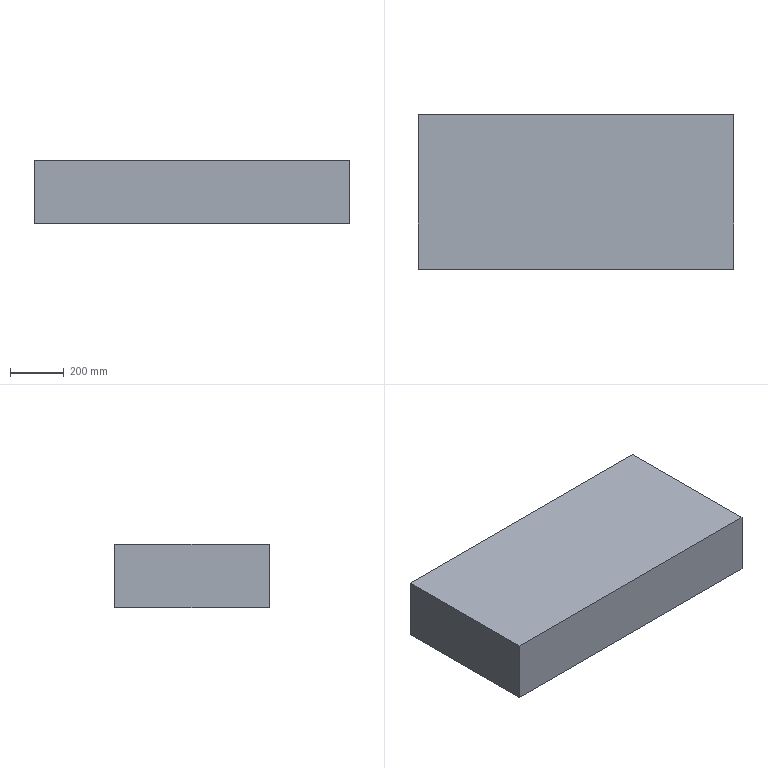Part | STEP file | 复件 Part 1^Upper罩 | 1 solid | 6 faces | box 1175 x 575 x 235 mm | volume 158771875 mm3 | plane 6
STEP:
#1=CARTESIAN_POINT('',(0.,0.,0.));
#2=DIRECTION('',(0.,0.,1.));
#3=DIRECTION('',(1.,0.,0.));
#4=AXIS2_PLACEMENT_3D('',#1,#2,#3);
#5=CARTESIAN_POINT('',(587.5,-287.5,0.));
#6=VERTEX_POINT('',#5);
#7=CARTESIAN_POINT('',(587.5,287.5,0.));
#8=VERTEX_POINT('',#7);
#9=CARTESIAN_POINT('',(587.5,287.5,0.));
#10=DIRECTION('',(0.,1.,0.));
#11=VECTOR('',#10,1.);
#12=LINE('',#9,#11);
#13=CARTESIAN_POINT('',(587.5,287.5,235.));
#14=DIRECTION('',(-1.,0.,0.));
#15=DIRECTION('',(0.,-1.,0.));
#16=AXIS2_PLACEMENT_3D('',#13,#14,#15);
#17=PLANE('',#16);
#18=CARTESIAN_POINT('',(0.,-235.));
#19=DIRECTION('',(-1.,0.));
#20=VECTOR('',#19,1.);
#21=LINE('',#18,#20);
#22=(GEOMETRIC_REPRESENTATION_CONTEXT(2)PARAMETRIC_REPRESENTATION_CONTEXT()REPRESENTATION_CONTEXT('',''));
#23=DEFINITIONAL_REPRESENTATION('',(#21),#22);
#24=PCURVE('',#17,#23);
#25=CARTESIAN_POINT('',(0.,0.,0.));
#26=DIRECTION('',(0.,0.,1.));
#27=DIRECTION('',(1.,0.,0.));
#28=AXIS2_PLACEMENT_3D('',#25,#26,#27);
#29=PLANE('',#28);
#30=CARTESIAN_POINT('',(587.5,287.5));
#31=DIRECTION('',(0.,1.));
#32=VECTOR('',#31,1.);
#33=LINE('',#30,#32);
#34=(GEOMETRIC_REPRESENTATION_CONTEXT(2)PARAMETRIC_REPRESENTATION_CONTEXT()REPRESENTATION_CONTEXT('',''));
#35=DEFINITIONAL_REPRESENTATION('',(#33),#34);
#36=PCURVE('',#29,#35);
#37=SURFACE_CURVE('',#12,(#24,#36),.PCURVE_S1.);
#38=EDGE_CURVE('',#6,#8,#37,.T.);
#39=ORIENTED_EDGE('',*,*,#38,.T.);
#40=CARTESIAN_POINT('',(587.5,287.5,235.));
#41=VERTEX_POINT('',#40);
#42=CARTESIAN_POINT('',(587.5,287.5,235.));
#43=DIRECTION('',(0.,0.,-1.));
#44=VECTOR('',#43,1.);
#45=LINE('',#42,#44);
#46=CARTESIAN_POINT('',(0.,0.));
#47=DIRECTION('',(0.,-1.));
#48=VECTOR('',#47,1.);
#49=LINE('',#46,#48);
#50=(GEOMETRIC_REPRESENTATION_CONTEXT(2)PARAMETRIC_REPRESENTATION_CONTEXT()REPRESENTATION_CONTEXT('',''));
#51=DEFINITIONAL_REPRESENTATION('',(#49),#50);
#52=PCURVE('',#17,#51);
#53=CARTESIAN_POINT('',(-587.5,287.5,235.));
#54=DIRECTION('',(0.,-1.,0.));
#55=DIRECTION('',(0.,0.,-1.));
#56=AXIS2_PLACEMENT_3D('',#53,#54,#55);
#57=PLANE('',#56);
#58=CARTESIAN_POINT('',(0.,1175.));
#59=DIRECTION('',(1.,0.));
#60=VECTOR('',#59,1.);
#61=LINE('',#58,#60);
#62=(GEOMETRIC_REPRESENTATION_CONTEXT(2)PARAMETRIC_REPRESENTATION_CONTEXT()REPRESENTATION_CONTEXT('',''));
#63=DEFINITIONAL_REPRESENTATION('',(#61),#62);
#64=PCURVE('',#57,#63);
#65=SURFACE_CURVE('',#45,(#52,#64),.PCURVE_S1.);
#66=EDGE_CURVE('',#41,#8,#65,.T.);
#67=ORIENTED_EDGE('',*,*,#66,.F.);
#68=CARTESIAN_POINT('',(587.5,-287.5,235.));
#69=VERTEX_POINT('',#68);
#70=CARTESIAN_POINT('',(587.5,287.5,235.));
#71=DIRECTION('',(0.,1.,0.));
#72=VECTOR('',#71,1.);
#73=LINE('',#70,#72);
#74=CARTESIAN_POINT('',(0.,0.));
#75=DIRECTION('',(-1.,0.));
#76=VECTOR('',#75,1.);
#77=LINE('',#74,#76);
#78=(GEOMETRIC_REPRESENTATION_CONTEXT(2)PARAMETRIC_REPRESENTATION_CONTEXT()REPRESENTATION_CONTEXT('',''));
#79=DEFINITIONAL_REPRESENTATION('',(#77),#78);
#80=PCURVE('',#17,#79);
#81=CARTESIAN_POINT('',(0.,0.,235.));
#82=DIRECTION('',(0.,0.,1.));
#83=DIRECTION('',(1.,0.,0.));
#84=AXIS2_PLACEMENT_3D('',#81,#82,#83);
#85=PLANE('',#84);
#86=CARTESIAN_POINT('',(587.5,287.5));
#87=DIRECTION('',(0.,1.));
#88=VECTOR('',#87,1.);
#89=LINE('',#86,#88);
#90=(GEOMETRIC_REPRESENTATION_CONTEXT(2)PARAMETRIC_REPRESENTATION_CONTEXT()REPRESENTATION_CONTEXT('',''));
#91=DEFINITIONAL_REPRESENTATION('',(#89),#90);
#92=PCURVE('',#85,#91);
#93=SURFACE_CURVE('',#73,(#80,#92),.PCURVE_S1.);
#94=EDGE_CURVE('',#69,#41,#93,.T.);
#95=ORIENTED_EDGE('',*,*,#94,.F.);
#96=CARTESIAN_POINT('',(587.5,-287.5,235.));
#97=DIRECTION('',(0.,0.,-1.));
#98=VECTOR('',#97,1.);
#99=LINE('',#96,#98);
#100=CARTESIAN_POINT('',(575.,0.));
#101=DIRECTION('',(0.,-1.));
#102=VECTOR('',#101,1.);
#103=LINE('',#100,#102);
#104=(GEOMETRIC_REPRESENTATION_CONTEXT(2)PARAMETRIC_REPRESENTATION_CONTEXT()REPRESENTATION_CONTEXT('',''));
#105=DEFINITIONAL_REPRESENTATION('',(#103),#104);
#106=PCURVE('',#17,#105);
#107=CARTESIAN_POINT('',(-587.5,-287.5,235.));
#108=DIRECTION('',(0.,1.,0.));
#109=DIRECTION('',(0.,0.,1.));
#110=AXIS2_PLACEMENT_3D('',#107,#108,#109);
#111=PLANE('',#110);
#112=CARTESIAN_POINT('',(0.,1175.));
#113=DIRECTION('',(-1.,0.));
#114=VECTOR('',#113,1.);
#115=LINE('',#112,#114);
#116=(GEOMETRIC_REPRESENTATION_CONTEXT(2)PARAMETRIC_REPRESENTATION_CONTEXT()REPRESENTATION_CONTEXT('',''));
#117=DEFINITIONAL_REPRESENTATION('',(#115),#116);
#118=PCURVE('',#111,#117);
#119=SURFACE_CURVE('',#99,(#106,#118),.PCURVE_S1.);
#120=EDGE_CURVE('',#69,#6,#119,.T.);
#121=ORIENTED_EDGE('',*,*,#120,.T.);
#122=EDGE_LOOP('',(#39,#67,#95,#121));
#123=FACE_BOUND('',#122,.T.);
#124=ADVANCED_FACE('',(#123),#17,.F.);
#125=CARTESIAN_POINT('',(-587.5,287.5,0.));
#126=VERTEX_POINT('',#125);
#127=CARTESIAN_POINT('',(-587.5,287.5,0.));
#128=DIRECTION('',(-1.,0.,0.));
#129=VECTOR('',#128,1.);
#130=LINE('',#127,#129);
#131=CARTESIAN_POINT('',(235.,0.));
#132=DIRECTION('',(0.,-1.));
#133=VECTOR('',#132,1.);
#134=LINE('',#131,#133);
#135=(GEOMETRIC_REPRESENTATION_CONTEXT(2)PARAMETRIC_REPRESENTATION_CONTEXT()REPRESENTATION_CONTEXT('',''));
#136=DEFINITIONAL_REPRESENTATION('',(#134),#135);
#137=PCURVE('',#57,#136);
#138=CARTESIAN_POINT('',(-587.5,287.5));
#139=DIRECTION('',(-1.,0.));
#140=VECTOR('',#139,1.);
#141=LINE('',#138,#140);
#142=(GEOMETRIC_REPRESENTATION_CONTEXT(2)PARAMETRIC_REPRESENTATION_CONTEXT()REPRESENTATION_CONTEXT('',''));
#143=DEFINITIONAL_REPRESENTATION('',(#141),#142);
#144=PCURVE('',#29,#143);
#145=SURFACE_CURVE('',#130,(#137,#144),.PCURVE_S1.);
#146=EDGE_CURVE('',#8,#126,#145,.T.);
#147=ORIENTED_EDGE('',*,*,#146,.T.);
#148=CARTESIAN_POINT('',(-587.5,287.5,235.));
#149=VERTEX_POINT('',#148);
#150=CARTESIAN_POINT('',(-587.5,287.5,235.));
#151=DIRECTION('',(0.,0.,-1.));
#152=VECTOR('',#151,1.);
#153=LINE('',#150,#152);
#154=CARTESIAN_POINT('',(0.,0.));
#155=DIRECTION('',(1.,0.));
#156=VECTOR('',#155,1.);
#157=LINE('',#154,#156);
#158=(GEOMETRIC_REPRESENTATION_CONTEXT(2)PARAMETRIC_REPRESENTATION_CONTEXT()REPRESENTATION_CONTEXT('',''));
#159=DEFINITIONAL_REPRESENTATION('',(#157),#158);
#160=PCURVE('',#57,#159);
#161=CARTESIAN_POINT('',(-587.5,287.5,235.));
#162=DIRECTION('',(1.,0.,0.));
#163=DIRECTION('',(0.,1.,0.));
#164=AXIS2_PLACEMENT_3D('',#161,#162,#163);
#165=PLANE('',#164);
#166=CARTESIAN_POINT('',(0.,0.));
#167=DIRECTION('',(0.,-1.));
#168=VECTOR('',#167,1.);
#169=LINE('',#166,#168);
#170=(GEOMETRIC_REPRESENTATION_CONTEXT(2)PARAMETRIC_REPRESENTATION_CONTEXT()REPRESENTATION_CONTEXT('',''));
#171=DEFINITIONAL_REPRESENTATION('',(#169),#170);
#172=PCURVE('',#165,#171);
#173=SURFACE_CURVE('',#153,(#160,#172),.PCURVE_S1.);
#174=EDGE_CURVE('',#149,#126,#173,.T.);
#175=ORIENTED_EDGE('',*,*,#174,.F.);
#176=CARTESIAN_POINT('',(-587.5,287.5,235.));
#177=DIRECTION('',(-1.,0.,0.));
#178=VECTOR('',#177,1.);
#179=LINE('',#176,#178);
#180=CARTESIAN_POINT('',(0.,0.));
#181=DIRECTION('',(0.,-1.));
#182=VECTOR('',#181,1.);
#183=LINE('',#180,#182);
#184=(GEOMETRIC_REPRESENTATION_CONTEXT(2)PARAMETRIC_REPRESENTATION_CONTEXT()REPRESENTATION_CONTEXT('',''));
#185=DEFINITIONAL_REPRESENTATION('',(#183),#184);
#186=PCURVE('',#57,#185);
#187=CARTESIAN_POINT('',(-587.5,287.5));
#188=DIRECTION('',(-1.,0.));
#189=VECTOR('',#188,1.);
#190=LINE('',#187,#189);
#191=(GEOMETRIC_REPRESENTATION_CONTEXT(2)PARAMETRIC_REPRESENTATION_CONTEXT()REPRESENTATION_CONTEXT('',''));
#192=DEFINITIONAL_REPRESENTATION('',(#190),#191);
#193=PCURVE('',#85,#192);
#194=SURFACE_CURVE('',#179,(#186,#193),.PCURVE_S1.);
#195=EDGE_CURVE('',#41,#149,#194,.T.);
#196=ORIENTED_EDGE('',*,*,#195,.F.);
#197=ORIENTED_EDGE('',*,*,#66,.T.);
#198=EDGE_LOOP('',(#147,#175,#196,#197));
#199=FACE_BOUND('',#198,.T.);
#200=ADVANCED_FACE('',(#199),#57,.F.);
#201=CARTESIAN_POINT('',(-587.5,-287.5,0.));
#202=VERTEX_POINT('',#201);
#203=CARTESIAN_POINT('',(-587.5,287.5,0.));
#204=DIRECTION('',(0.,-1.,0.));
#205=VECTOR('',#204,1.);
#206=LINE('',#203,#205);
#207=CARTESIAN_POINT('',(0.,-235.));
#208=DIRECTION('',(-1.,0.));
#209=VECTOR('',#208,1.);
#210=LINE('',#207,#209);
#211=(GEOMETRIC_REPRESENTATION_CONTEXT(2)PARAMETRIC_REPRESENTATION_CONTEXT()REPRESENTATION_CONTEXT('',''));
#212=DEFINITIONAL_REPRESENTATION('',(#210),#211);
#213=PCURVE('',#165,#212);
#214=CARTESIAN_POINT('',(-587.5,287.5));
#215=DIRECTION('',(0.,-1.));
#216=VECTOR('',#215,1.);
#217=LINE('',#214,#216);
#218=(GEOMETRIC_REPRESENTATION_CONTEXT(2)PARAMETRIC_REPRESENTATION_CONTEXT()REPRESENTATION_CONTEXT('',''));
#219=DEFINITIONAL_REPRESENTATION('',(#217),#218);
#220=PCURVE('',#29,#219);
#221=SURFACE_CURVE('',#206,(#213,#220),.PCURVE_S1.);
#222=EDGE_CURVE('',#126,#202,#221,.T.);
#223=ORIENTED_EDGE('',*,*,#222,.T.);
#224=CARTESIAN_POINT('',(-587.5,-287.5,235.));
#225=VERTEX_POINT('',#224);
#226=CARTESIAN_POINT('',(-587.5,-287.5,235.));
#227=DIRECTION('',(0.,0.,-1.));
#228=VECTOR('',#227,1.);
#229=LINE('',#226,#228);
#230=CARTESIAN_POINT('',(-575.,0.));
#231=DIRECTION('',(0.,-1.));
#232=VECTOR('',#231,1.);
#233=LINE('',#230,#232);
#234=(GEOMETRIC_REPRESENTATION_CONTEXT(2)PARAMETRIC_REPRESENTATION_CONTEXT()REPRESENTATION_CONTEXT('',''));
#235=DEFINITIONAL_REPRESENTATION('',(#233),#234);
#236=PCURVE('',#165,#235);
#237=CARTESIAN_POINT('',(0.,0.));
#238=DIRECTION('',(-1.,0.));
#239=VECTOR('',#238,1.);
#240=LINE('',#237,#239);
#241=(GEOMETRIC_REPRESENTATION_CONTEXT(2)PARAMETRIC_REPRESENTATION_CONTEXT()REPRESENTATION_CONTEXT('',''));
#242=DEFINITIONAL_REPRESENTATION('',(#240),#241);
#243=PCURVE('',#111,#242);
#244=SURFACE_CURVE('',#229,(#236,#243),.PCURVE_S1.);
#245=EDGE_CURVE('',#225,#202,#244,.T.);
#246=ORIENTED_EDGE('',*,*,#245,.F.);
#247=CARTESIAN_POINT('',(-587.5,287.5,235.));
#248=DIRECTION('',(0.,-1.,0.));
#249=VECTOR('',#248,1.);
#250=LINE('',#247,#249);
#251=CARTESIAN_POINT('',(0.,0.));
#252=DIRECTION('',(-1.,0.));
#253=VECTOR('',#252,1.);
#254=LINE('',#251,#253);
#255=(GEOMETRIC_REPRESENTATION_CONTEXT(2)PARAMETRIC_REPRESENTATION_CONTEXT()REPRESENTATION_CONTEXT('',''));
#256=DEFINITIONAL_REPRESENTATION('',(#254),#255);
#257=PCURVE('',#165,#256);
#258=CARTESIAN_POINT('',(-587.5,287.5));
#259=DIRECTION('',(0.,-1.));
#260=VECTOR('',#259,1.);
#261=LINE('',#258,#260);
#262=(GEOMETRIC_REPRESENTATION_CONTEXT(2)PARAMETRIC_REPRESENTATION_CONTEXT()REPRESENTATION_CONTEXT('',''));
#263=DEFINITIONAL_REPRESENTATION('',(#261),#262);
#264=PCURVE('',#85,#263);
#265=SURFACE_CURVE('',#250,(#257,#264),.PCURVE_S1.);
#266=EDGE_CURVE('',#149,#225,#265,.T.);
#267=ORIENTED_EDGE('',*,*,#266,.F.);
#268=ORIENTED_EDGE('',*,*,#174,.T.);
#269=EDGE_LOOP('',(#223,#246,#267,#268));
#270=FACE_BOUND('',#269,.T.);
#271=ADVANCED_FACE('',(#270),#165,.F.);
#272=CARTESIAN_POINT('',(-587.5,-287.5,0.));
#273=DIRECTION('',(1.,0.,0.));
#274=VECTOR('',#273,1.);
#275=LINE('',#272,#274);
#276=CARTESIAN_POINT('',(-235.,0.));
#277=DIRECTION('',(0.,1.));
#278=VECTOR('',#277,1.);
#279=LINE('',#276,#278);
#280=(GEOMETRIC_REPRESENTATION_CONTEXT(2)PARAMETRIC_REPRESENTATION_CONTEXT()REPRESENTATION_CONTEXT('',''));
#281=DEFINITIONAL_REPRESENTATION('',(#279),#280);
#282=PCURVE('',#111,#281);
#283=CARTESIAN_POINT('',(-587.5,-287.5));
#284=DIRECTION('',(1.,0.));
#285=VECTOR('',#284,1.);
#286=LINE('',#283,#285);
#287=(GEOMETRIC_REPRESENTATION_CONTEXT(2)PARAMETRIC_REPRESENTATION_CONTEXT()REPRESENTATION_CONTEXT('',''));
#288=DEFINITIONAL_REPRESENTATION('',(#286),#287);
#289=PCURVE('',#29,#288);
#290=SURFACE_CURVE('',#275,(#282,#289),.PCURVE_S1.);
#291=EDGE_CURVE('',#202,#6,#290,.T.);
#292=ORIENTED_EDGE('',*,*,#291,.T.);
#293=ORIENTED_EDGE('',*,*,#120,.F.);
#294=CARTESIAN_POINT('',(-587.5,-287.5,235.));
#295=DIRECTION('',(1.,0.,0.));
#296=VECTOR('',#295,1.);
#297=LINE('',#294,#296);
#298=CARTESIAN_POINT('',(0.,0.));
#299=DIRECTION('',(0.,1.));
#300=VECTOR('',#299,1.);
#301=LINE('',#298,#300);
#302=(GEOMETRIC_REPRESENTATION_CONTEXT(2)PARAMETRIC_REPRESENTATION_CONTEXT()REPRESENTATION_CONTEXT('',''));
#303=DEFINITIONAL_REPRESENTATION('',(#301),#302);
#304=PCURVE('',#111,#303);
#305=CARTESIAN_POINT('',(-587.5,-287.5));
#306=DIRECTION('',(1.,0.));
#307=VECTOR('',#306,1.);
#308=LINE('',#305,#307);
#309=(GEOMETRIC_REPRESENTATION_CONTEXT(2)PARAMETRIC_REPRESENTATION_CONTEXT()REPRESENTATION_CONTEXT('',''));
#310=DEFINITIONAL_REPRESENTATION('',(#308),#309);
#311=PCURVE('',#85,#310);
#312=SURFACE_CURVE('',#297,(#304,#311),.PCURVE_S1.);
#313=EDGE_CURVE('',#225,#69,#312,.T.);
#314=ORIENTED_EDGE('',*,*,#313,.F.);
#315=ORIENTED_EDGE('',*,*,#245,.T.);
#316=EDGE_LOOP('',(#292,#293,#314,#315));
#317=FACE_BOUND('',#316,.T.);
#318=ADVANCED_FACE('',(#317),#111,.F.);
#319=ORIENTED_EDGE('',*,*,#94,.T.);
#320=ORIENTED_EDGE('',*,*,#195,.T.);
#321=ORIENTED_EDGE('',*,*,#266,.T.);
#322=ORIENTED_EDGE('',*,*,#313,.T.);
#323=EDGE_LOOP('',(#319,#320,#321,#322));
#324=FACE_BOUND('',#323,.T.);
#325=ADVANCED_FACE('',(#324),#85,.T.);
#326=ORIENTED_EDGE('',*,*,#38,.F.);
#327=ORIENTED_EDGE('',*,*,#291,.F.);
#328=ORIENTED_EDGE('',*,*,#222,.F.);
#329=ORIENTED_EDGE('',*,*,#146,.F.);
#330=EDGE_LOOP('',(#326,#327,#328,#329));
#331=FACE_BOUND('',#330,.T.);
#332=ADVANCED_FACE('',(#331),#29,.F.);
#333=CLOSED_SHELL('',(#124,#200,#271,#318,#325,#332));
#334=MANIFOLD_SOLID_BREP('',#333);
#335=(LENGTH_UNIT()NAMED_UNIT(*)SI_UNIT(.MILLI.,.METRE.));
#336=UNCERTAINTY_MEASURE_WITH_UNIT(LENGTH_MEASURE(0.0000001),#335,'','');
#337=(NAMED_UNIT(*)PLANE_ANGLE_UNIT()SI_UNIT($,.RADIAN.));
#338=(NAMED_UNIT(*)SI_UNIT($,.STERADIAN.)SOLID_ANGLE_UNIT());
#339=(GEOMETRIC_REPRESENTATION_CONTEXT(3)GLOBAL_UNCERTAINTY_ASSIGNED_CONTEXT((#336))GLOBAL_UNIT_ASSIGNED_CONTEXT((#335,#337,#338))REPRESENTATION_CONTEXT('',''));
#340=ADVANCED_BREP_SHAPE_REPRESENTATION('',(#4,#334),#339);